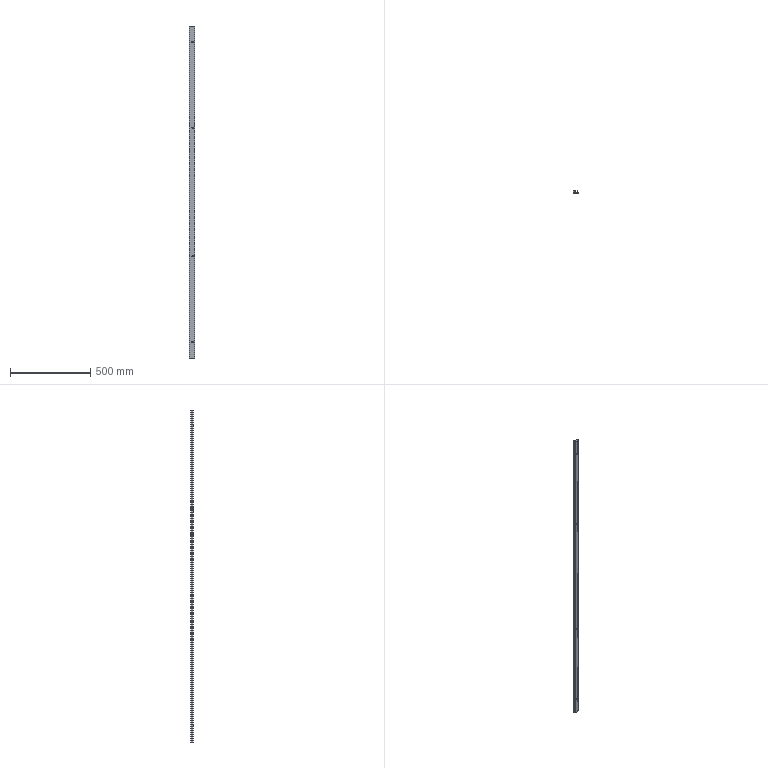Part | SolidWorks | features ICE 2, BaseBody 1, HoleWzd 1, MoveFace 1 | 1 solid | 35 faces | box 33.5 x 13.5 x 2066 mm | volume 386658 mm3 | plane 17 | cylinder 10 | cone 8 | commonest cylinder face diameters 13.44 x4 2 x3 4 x2 1.5 x1
STEP:
#1=CARTESIAN_POINT('',(20.,0.,1869.72));
#2=VERTEX_POINT('',#1);
#3=CARTESIAN_POINT('',(20.,0.,1862.28));
#4=VERTEX_POINT('',#3);
#5=CARTESIAN_POINT('',(20.,0.,1866.));
#6=DIRECTION('',(0.,-1.,0.));
#7=DIRECTION('',(0.,0.,-1.));
#8=AXIS2_PLACEMENT_3D('',#5,#6,#7);
#9=CIRCLE('',#8,3.72);
#10=EDGE_CURVE('',#2,#4,#9,.T.);
#11=ORIENTED_EDGE('',*,*,#10,.T.);
#12=CARTESIAN_POINT('',(20.,3.,1859.28));
#13=VERTEX_POINT('',#12);
#14=CARTESIAN_POINT('',(20.,3.,1859.28));
#15=DIRECTION('',(0.,0.7071,-0.7071));
#16=VECTOR('',#15,1000.);
#17=LINE('',#14,#16);
#18=EDGE_CURVE('',#4,#13,#17,.T.);
#19=ORIENTED_EDGE('',*,*,#18,.T.);
#20=CARTESIAN_POINT('',(20.,3.,1872.72));
#21=VERTEX_POINT('',#20);
#22=CARTESIAN_POINT('',(20.,3.,1866.));
#23=DIRECTION('',(0.,1.,0.));
#24=DIRECTION('',(0.,0.,1.));
#25=AXIS2_PLACEMENT_3D('',#22,#23,#24);
#26=CIRCLE('',#25,6.72);
#27=EDGE_CURVE('',#13,#21,#26,.T.);
#28=ORIENTED_EDGE('',*,*,#27,.T.);
#29=CARTESIAN_POINT('',(20.,3.,1872.72));
#30=DIRECTION('',(0.,0.7071,0.7071));
#31=VECTOR('',#30,1000.);
#32=LINE('',#29,#31);
#33=EDGE_CURVE('',#2,#21,#32,.T.);
#34=ORIENTED_EDGE('',*,*,#33,.F.);
#35=EDGE_LOOP('',(#11,#19,#28,#34));
#36=FACE_OUTER_BOUND('',#35,.T.);
#37=CARTESIAN_POINT('',(20.,3.,1866.));
#38=DIRECTION('',(0.,1.,0.));
#39=DIRECTION('',(0.,0.,1.));
#40=AXIS2_PLACEMENT_3D('',#37,#38,#39);
#41=CONICAL_SURFACE('',#40,6.72,0.7854);
#42=ADVANCED_FACE('',(#36),#41,.F.);
#43=CARTESIAN_POINT('',(20.,0.,3.72));
#44=VERTEX_POINT('',#43);
#45=CARTESIAN_POINT('',(20.,0.,-3.72));
#46=VERTEX_POINT('',#45);
#47=CARTESIAN_POINT('',(20.,0.,0.));
#48=DIRECTION('',(0.,-1.,0.));
#49=DIRECTION('',(0.,0.,-1.));
#50=AXIS2_PLACEMENT_3D('',#47,#48,#49);
#51=CIRCLE('',#50,3.72);
#52=EDGE_CURVE('',#44,#46,#51,.T.);
#53=ORIENTED_EDGE('',*,*,#52,.T.);
#54=CARTESIAN_POINT('',(20.,3.,-6.72));
#55=VERTEX_POINT('',#54);
#56=CARTESIAN_POINT('',(20.,3.,-6.72));
#57=DIRECTION('',(0.,0.7071,-0.7071));
#58=VECTOR('',#57,1000.);
#59=LINE('',#56,#58);
#60=EDGE_CURVE('',#46,#55,#59,.T.);
#61=ORIENTED_EDGE('',*,*,#60,.T.);
#62=CARTESIAN_POINT('',(20.,3.,6.72));
#63=VERTEX_POINT('',#62);
#64=CARTESIAN_POINT('',(20.,3.,0.));
#65=DIRECTION('',(0.,1.,0.));
#66=DIRECTION('',(0.,0.,1.));
#67=AXIS2_PLACEMENT_3D('',#64,#65,#66);
#68=CIRCLE('',#67,6.72);
#69=EDGE_CURVE('',#55,#63,#68,.T.);
#70=ORIENTED_EDGE('',*,*,#69,.T.);
#71=CARTESIAN_POINT('',(20.,3.,6.72));
#72=DIRECTION('',(0.,0.7071,0.7071));
#73=VECTOR('',#72,1000.);
#74=LINE('',#71,#73);
#75=EDGE_CURVE('',#44,#63,#74,.T.);
#76=ORIENTED_EDGE('',*,*,#75,.F.);
#77=EDGE_LOOP('',(#53,#61,#70,#76));
#78=FACE_OUTER_BOUND('',#77,.T.);
#79=CARTESIAN_POINT('',(20.,3.,0.));
#80=DIRECTION('',(0.,1.,0.));
#81=DIRECTION('',(0.,0.,1.));
#82=AXIS2_PLACEMENT_3D('',#79,#80,#81);
#83=CONICAL_SURFACE('',#82,6.72,0.7854);
#84=ADVANCED_FACE('',(#78),#83,.F.);
#85=CARTESIAN_POINT('',(20.,0.,536.72));
#86=VERTEX_POINT('',#85);
#87=CARTESIAN_POINT('',(20.,0.,529.28));
#88=VERTEX_POINT('',#87);
#89=CARTESIAN_POINT('',(20.,0.,533.));
#90=DIRECTION('',(0.,-1.,0.));
#91=DIRECTION('',(0.,0.,-1.));
#92=AXIS2_PLACEMENT_3D('',#89,#90,#91);
#93=CIRCLE('',#92,3.72);
#94=EDGE_CURVE('',#86,#88,#93,.T.);
#95=ORIENTED_EDGE('',*,*,#94,.T.);
#96=CARTESIAN_POINT('',(20.,3.,526.28));
#97=VERTEX_POINT('',#96);
#98=CARTESIAN_POINT('',(20.,3.,526.28));
#99=DIRECTION('',(0.,0.7071,-0.7071));
#100=VECTOR('',#99,1000.);
#101=LINE('',#98,#100);
#102=EDGE_CURVE('',#88,#97,#101,.T.);
#103=ORIENTED_EDGE('',*,*,#102,.T.);
#104=CARTESIAN_POINT('',(20.,3.,539.72));
#105=VERTEX_POINT('',#104);
#106=CARTESIAN_POINT('',(20.,3.,533.));
#107=DIRECTION('',(0.,1.,0.));
#108=DIRECTION('',(0.,0.,1.));
#109=AXIS2_PLACEMENT_3D('',#106,#107,#108);
#110=CIRCLE('',#109,6.72);
#111=EDGE_CURVE('',#97,#105,#110,.T.);
#112=ORIENTED_EDGE('',*,*,#111,.T.);
#113=CARTESIAN_POINT('',(20.,3.,539.72));
#114=DIRECTION('',(0.,0.7071,0.7071));
#115=VECTOR('',#114,1000.);
#116=LINE('',#113,#115);
#117=EDGE_CURVE('',#86,#105,#116,.T.);
#118=ORIENTED_EDGE('',*,*,#117,.F.);
#119=EDGE_LOOP('',(#95,#103,#112,#118));
#120=FACE_OUTER_BOUND('',#119,.T.);
#121=CARTESIAN_POINT('',(20.,3.,533.));
#122=DIRECTION('',(0.,1.,0.));
#123=DIRECTION('',(0.,0.,1.));
#124=AXIS2_PLACEMENT_3D('',#121,#122,#123);
#125=CONICAL_SURFACE('',#124,6.72,0.7854);
#126=ADVANCED_FACE('',(#120),#125,.F.);
#127=CARTESIAN_POINT('',(20.,0.,1336.72));
#128=VERTEX_POINT('',#127);
#129=CARTESIAN_POINT('',(20.,0.,1329.28));
#130=VERTEX_POINT('',#129);
#131=CARTESIAN_POINT('',(20.,0.,1333.));
#132=DIRECTION('',(0.,-1.,0.));
#133=DIRECTION('',(0.,0.,-1.));
#134=AXIS2_PLACEMENT_3D('',#131,#132,#133);
#135=CIRCLE('',#134,3.72);
#136=EDGE_CURVE('',#128,#130,#135,.T.);
#137=ORIENTED_EDGE('',*,*,#136,.T.);
#138=CARTESIAN_POINT('',(20.,3.,1326.28));
#139=VERTEX_POINT('',#138);
#140=CARTESIAN_POINT('',(20.,3.,1326.28));
#141=DIRECTION('',(0.,0.7071,-0.7071));
#142=VECTOR('',#141,1000.);
#143=LINE('',#140,#142);
#144=EDGE_CURVE('',#130,#139,#143,.T.);
#145=ORIENTED_EDGE('',*,*,#144,.T.);
#146=CARTESIAN_POINT('',(20.,3.,1339.72));
#147=VERTEX_POINT('',#146);
#148=CARTESIAN_POINT('',(20.,3.,1333.));
#149=DIRECTION('',(0.,1.,0.));
#150=DIRECTION('',(0.,0.,1.));
#151=AXIS2_PLACEMENT_3D('',#148,#149,#150);
#152=CIRCLE('',#151,6.72);
#153=EDGE_CURVE('',#139,#147,#152,.T.);
#154=ORIENTED_EDGE('',*,*,#153,.T.);
#155=CARTESIAN_POINT('',(20.,3.,1339.72));
#156=DIRECTION('',(0.,0.7071,0.7071));
#157=VECTOR('',#156,1000.);
#158=LINE('',#155,#157);
#159=EDGE_CURVE('',#128,#147,#158,.T.);
#160=ORIENTED_EDGE('',*,*,#159,.F.);
#161=EDGE_LOOP('',(#137,#145,#154,#160));
#162=FACE_OUTER_BOUND('',#161,.T.);
#163=CARTESIAN_POINT('',(20.,3.,1333.));
#164=DIRECTION('',(0.,1.,0.));
#165=DIRECTION('',(0.,0.,1.));
#166=AXIS2_PLACEMENT_3D('',#163,#164,#165);
#167=CONICAL_SURFACE('',#166,6.72,0.7854);
#168=ADVANCED_FACE('',(#162),#167,.F.);
#169=CARTESIAN_POINT('',(24.5,10.5,1328.009));
#170=VERTEX_POINT('',#169);
#171=CARTESIAN_POINT('',(24.5,3.,1328.009));
#172=VERTEX_POINT('',#171);
#173=CARTESIAN_POINT('',(24.5,64.,1328.009));
#174=DIRECTION('',(0.,-1.,0.));
#175=VECTOR('',#174,1000.);
#176=LINE('',#173,#175);
#177=EDGE_CURVE('',#170,#172,#176,.T.);
#178=ORIENTED_EDGE('',*,*,#177,.F.);
#179=CARTESIAN_POINT('',(24.5,10.5,537.991));
#180=VERTEX_POINT('',#179);
#181=CARTESIAN_POINT('',(24.5,10.5,-100.));
#182=DIRECTION('',(0.,0.,-1.));
#183=VECTOR('',#182,1000.);
#184=LINE('',#181,#183);
#185=EDGE_CURVE('',#170,#180,#184,.T.);
#186=ORIENTED_EDGE('',*,*,#185,.T.);
#187=CARTESIAN_POINT('',(24.5,3.,537.991));
#188=VERTEX_POINT('',#187);
#189=CARTESIAN_POINT('',(24.5,13.5,537.991));
#190=DIRECTION('',(0.,-1.,0.));
#191=VECTOR('',#190,1000.);
#192=LINE('',#189,#191);
#193=EDGE_CURVE('',#180,#188,#192,.T.);
#194=ORIENTED_EDGE('',*,*,#193,.T.);
#195=CARTESIAN_POINT('',(24.5,3.,-100.));
#196=DIRECTION('',(0.,0.,-1.));
#197=VECTOR('',#196,1000.);
#198=LINE('',#195,#197);
#199=EDGE_CURVE('',#172,#188,#198,.T.);
#200=ORIENTED_EDGE('',*,*,#199,.F.);
#201=EDGE_LOOP('',(#178,#186,#194,#200));
#202=FACE_OUTER_BOUND('',#201,.T.);
#203=CARTESIAN_POINT('',(24.5,10.5,-100.));
#204=DIRECTION('',(-1.,0.,0.));
#205=DIRECTION('',(0.,0.,1.));
#206=AXIS2_PLACEMENT_3D('',#203,#204,#205);
#207=PLANE('',#206);
#208=ADVANCED_FACE('',(#202),#207,.T.);
#209=CARTESIAN_POINT('',(24.5,10.5,1337.991));
#210=VERTEX_POINT('',#209);
#211=CARTESIAN_POINT('',(24.5,10.5,1337.991));
#212=CARTESIAN_POINT('',(24.5,10.64,1337.991));
#213=CARTESIAN_POINT('',(24.514,10.776,1337.978));
#214=CARTESIAN_POINT('',(24.57,11.042,1337.927));
#215=CARTESIAN_POINT('',(24.611,11.171,1337.889));
#216=CARTESIAN_POINT('',(24.713,11.408,1337.791));
#217=CARTESIAN_POINT('',(24.775,11.519,1337.73));
#218=CARTESIAN_POINT('',(24.908,11.717,1337.591));
#219=CARTESIAN_POINT('',(24.981,11.806,1337.512));
#220=CARTESIAN_POINT('',(25.207,12.042,1337.254));
#221=CARTESIAN_POINT('',(25.363,12.155,1337.058));
#222=CARTESIAN_POINT('',(25.665,12.326,1336.624));
#223=CARTESIAN_POINT('',(25.806,12.38,1336.395));
#224=CARTESIAN_POINT('',(26.061,12.456,1335.916));
#225=CARTESIAN_POINT('',(26.176,12.476,1335.663));
#226=CARTESIAN_POINT('',(26.372,12.498,1335.151));
#227=CARTESIAN_POINT('',(26.454,12.501,1334.891));
#228=CARTESIAN_POINT('',(26.586,12.499,1334.362));
#229=CARTESIAN_POINT('',(26.636,12.496,1334.093));
#230=CARTESIAN_POINT('',(26.703,12.49,1333.547));
#231=CARTESIAN_POINT('',(26.72,12.488,1333.271));
#232=CARTESIAN_POINT('',(26.72,12.488,1332.725));
#233=CARTESIAN_POINT('',(26.703,12.49,1332.453));
#234=CARTESIAN_POINT('',(26.637,12.496,1331.911));
#235=CARTESIAN_POINT('',(26.587,12.499,1331.64));
#236=CARTESIAN_POINT('',(26.387,12.501,1330.839));
#237=CARTESIAN_POINT('',(26.191,12.494,1330.329));
#238=CARTESIAN_POINT('',(25.805,12.38,1329.604));
#239=CARTESIAN_POINT('',(25.663,12.325,1329.373));
#240=CARTESIAN_POINT('',(25.364,12.155,1328.943));
#241=CARTESIAN_POINT('',(25.205,12.039,1328.744));
#242=CARTESIAN_POINT('',(24.981,11.805,1328.488));
#243=CARTESIAN_POINT('',(24.907,11.716,1328.408));
#244=CARTESIAN_POINT('',(24.774,11.518,1328.27));
#245=CARTESIAN_POINT('',(24.714,11.409,1328.21));
#246=CARTESIAN_POINT('',(24.611,11.17,1328.111));
#247=CARTESIAN_POINT('',(24.571,11.044,1328.074));
#248=CARTESIAN_POINT('',(24.515,10.78,1328.023));
#249=CARTESIAN_POINT('',(24.5,10.64,1328.009));
#250=CARTESIAN_POINT('',(24.5,10.5,1328.009));
#251=B_SPLINE_CURVE_WITH_KNOTS('',3,(#211,#212,#213,#214,#215,#216,#217,#218,#219,#220,#221,#222,#223,#224,#225,#226,#227,#228,#229,#230,#231,#232,#233,#234,#235,#236,#237,#238,#239,#240,#241,#242,#243,#244,#245,#246,#247,#248,#249,#250),.UNSPECIFIED.,.F.,.F.,(4,2,2,2,2,2,2,2,2,2,2,2,2,2,2,2,2,2,2,4),(0.,0.0004127,0.0008255,0.001238,0.001651,0.002476,0.003302,0.004127,0.004953,0.005778,0.006604,0.007429,0.008255,0.009906,0.01073,0.01156,0.01197,0.01238,0.01279,0.01321),.UNSPECIFIED.);
#252=EDGE_CURVE('',#210,#170,#251,.T.);
#253=ORIENTED_EDGE('',*,*,#252,.F.);
#254=CARTESIAN_POINT('',(24.5,10.5,1861.009));
#255=VERTEX_POINT('',#254);
#256=CARTESIAN_POINT('',(24.5,10.5,-100.));
#257=DIRECTION('',(0.,0.,-1.));
#258=VECTOR('',#257,1000.);
#259=LINE('',#256,#258);
#260=EDGE_CURVE('',#255,#210,#259,.T.);
#261=ORIENTED_EDGE('',*,*,#260,.F.);
#262=CARTESIAN_POINT('',(24.5,10.5,1870.991));
#263=VERTEX_POINT('',#262);
#264=CARTESIAN_POINT('',(24.5,10.5,1861.009));
#265=CARTESIAN_POINT('',(24.5,10.64,1861.009));
#266=CARTESIAN_POINT('',(24.514,10.776,1861.022));
#267=CARTESIAN_POINT('',(24.57,11.042,1861.073));
#268=CARTESIAN_POINT('',(24.611,11.171,1861.111));
#269=CARTESIAN_POINT('',(24.713,11.408,1861.209));
#270=CARTESIAN_POINT('',(24.775,11.519,1861.27));
#271=CARTESIAN_POINT('',(24.908,11.717,1861.409));
#272=CARTESIAN_POINT('',(24.981,11.806,1861.488));
#273=CARTESIAN_POINT('',(25.207,12.042,1861.746));
#274=CARTESIAN_POINT('',(25.363,12.155,1861.942));
#275=CARTESIAN_POINT('',(25.665,12.326,1862.376));
#276=CARTESIAN_POINT('',(25.806,12.38,1862.605));
#277=CARTESIAN_POINT('',(26.061,12.456,1863.084));
#278=CARTESIAN_POINT('',(26.176,12.476,1863.337));
#279=CARTESIAN_POINT('',(26.372,12.498,1863.849));
#280=CARTESIAN_POINT('',(26.454,12.501,1864.109));
#281=CARTESIAN_POINT('',(26.586,12.499,1864.638));
#282=CARTESIAN_POINT('',(26.636,12.496,1864.907));
#283=CARTESIAN_POINT('',(26.703,12.49,1865.453));
#284=CARTESIAN_POINT('',(26.72,12.488,1865.729));
#285=CARTESIAN_POINT('',(26.72,12.488,1866.275));
#286=CARTESIAN_POINT('',(26.703,12.49,1866.547));
#287=CARTESIAN_POINT('',(26.637,12.496,1867.089));
#288=CARTESIAN_POINT('',(26.587,12.499,1867.36));
#289=CARTESIAN_POINT('',(26.387,12.501,1868.161));
#290=CARTESIAN_POINT('',(26.191,12.494,1868.671));
#291=CARTESIAN_POINT('',(25.805,12.38,1869.396));
#292=CARTESIAN_POINT('',(25.663,12.325,1869.627));
#293=CARTESIAN_POINT('',(25.364,12.155,1870.057));
#294=CARTESIAN_POINT('',(25.205,12.039,1870.256));
#295=CARTESIAN_POINT('',(24.981,11.805,1870.512));
#296=CARTESIAN_POINT('',(24.907,11.716,1870.592));
#297=CARTESIAN_POINT('',(24.774,11.518,1870.73));
#298=CARTESIAN_POINT('',(24.714,11.409,1870.79));
#299=CARTESIAN_POINT('',(24.611,11.17,1870.889));
#300=CARTESIAN_POINT('',(24.571,11.044,1870.926));
#301=CARTESIAN_POINT('',(24.515,10.78,1870.977));
#302=CARTESIAN_POINT('',(24.5,10.64,1870.991));
#303=CARTESIAN_POINT('',(24.5,10.5,1870.991));
#304=B_SPLINE_CURVE_WITH_KNOTS('',3,(#264,#265,#266,#267,#268,#269,#270,#271,#272,#273,#274,#275,#276,#277,#278,#279,#280,#281,#282,#283,#284,#285,#286,#287,#288,#289,#290,#291,#292,#293,#294,#295,#296,#297,#298,#299,#300,#301,#302,#303),.UNSPECIFIED.,.F.,.F.,(4,2,2,2,2,2,2,2,2,2,2,2,2,2,2,2,2,2,2,4),(0.,0.0004127,0.0008255,0.001238,0.001651,0.002476,0.003302,0.004127,0.004953,0.005778,0.006604,0.007429,0.008255,0.009906,0.01073,0.01156,0.01197,0.01238,0.01279,0.01321),.UNSPECIFIED.);
#305=EDGE_CURVE('',#255,#263,#304,.T.);
#306=ORIENTED_EDGE('',*,*,#305,.T.);
#307=CARTESIAN_POINT('',(24.5,10.5,1966.));
#308=VERTEX_POINT('',#307);
#309=CARTESIAN_POINT('',(24.5,10.5,-100.));
#310=DIRECTION('',(0.,0.,-1.));
#311=VECTOR('',#310,1000.);
#312=LINE('',#309,#311);
#313=EDGE_CURVE('',#308,#263,#312,.T.);
#314=ORIENTED_EDGE('',*,*,#313,.F.);
#315=CARTESIAN_POINT('',(28.5,10.5,1966.));
#316=VERTEX_POINT('',#315);
#317=CARTESIAN_POINT('',(26.5,10.5,1966.));
#318=DIRECTION('',(0.,0.,1.));
#319=DIRECTION('',(1.,0.,0.));
#320=AXIS2_PLACEMENT_3D('',#317,#318,#319);
#321=CIRCLE('',#320,2.);
#322=EDGE_CURVE('',#316,#308,#321,.T.);
#323=ORIENTED_EDGE('',*,*,#322,.F.);
#324=CARTESIAN_POINT('',(28.5,10.5,-100.));
#325=VERTEX_POINT('',#324);
#326=CARTESIAN_POINT('',(28.5,10.5,-100.));
#327=DIRECTION('',(0.,0.,-1.));
#328=VECTOR('',#327,1000.);
#329=LINE('',#326,#328);
#330=EDGE_CURVE('',#316,#325,#329,.T.);
#331=ORIENTED_EDGE('',*,*,#330,.T.);
#332=CARTESIAN_POINT('',(24.5,10.5,-100.));
#333=VERTEX_POINT('',#332);
#334=CARTESIAN_POINT('',(26.5,10.5,-100.));
#335=DIRECTION('',(0.,0.,1.));
#336=DIRECTION('',(-1.,0.,0.));
#337=AXIS2_PLACEMENT_3D('',#334,#335,#336);
#338=CIRCLE('',#337,2.);
#339=EDGE_CURVE('',#325,#333,#338,.T.);
#340=ORIENTED_EDGE('',*,*,#339,.T.);
#341=CARTESIAN_POINT('',(24.5,10.5,-4.991));
#342=VERTEX_POINT('',#341);
#343=CARTESIAN_POINT('',(24.5,10.5,-100.));
#344=DIRECTION('',(0.,0.,-1.));
#345=VECTOR('',#344,1000.);
#346=LINE('',#343,#345);
#347=EDGE_CURVE('',#342,#333,#346,.T.);
#348=ORIENTED_EDGE('',*,*,#347,.F.);
#349=CARTESIAN_POINT('',(24.5,10.5,4.991));
#350=VERTEX_POINT('',#349);
#351=CARTESIAN_POINT('',(24.5,10.5,-4.991));
#352=CARTESIAN_POINT('',(24.5,10.638,-4.991));
#353=CARTESIAN_POINT('',(24.515,10.777,-4.978));
#354=CARTESIAN_POINT('',(24.57,11.043,-4.927));
#355=CARTESIAN_POINT('',(24.611,11.171,-4.889));
#356=CARTESIAN_POINT('',(24.765,11.529,-4.74));
#357=CARTESIAN_POINT('',(24.907,11.728,-4.597));
#358=CARTESIAN_POINT('',(25.205,12.04,-4.256));
#359=CARTESIAN_POINT('',(25.365,12.156,-4.055));
#360=CARTESIAN_POINT('',(25.663,12.325,-3.627));
#361=CARTESIAN_POINT('',(25.806,12.38,-3.395));
#362=CARTESIAN_POINT('',(26.19,12.494,-2.672));
#363=CARTESIAN_POINT('',(26.387,12.501,-2.161));
#364=CARTESIAN_POINT('',(26.654,12.499,-1.091));
#365=CARTESIAN_POINT('',(26.72,12.488,-0.5481));
#366=CARTESIAN_POINT('',(26.72,12.488,0.2773));
#367=CARTESIAN_POINT('',(26.703,12.49,0.5529));
#368=CARTESIAN_POINT('',(26.636,12.496,1.095));
#369=CARTESIAN_POINT('',(26.586,12.499,1.362));
#370=CARTESIAN_POINT('',(26.388,12.501,2.155));
#371=CARTESIAN_POINT('',(26.188,12.493,2.677));
#372=CARTESIAN_POINT('',(25.805,12.38,3.396));
#373=CARTESIAN_POINT('',(25.662,12.324,3.629));
#374=CARTESIAN_POINT('',(25.438,12.197,3.95));
#375=CARTESIAN_POINT('',(25.362,12.147,4.053));
#376=CARTESIAN_POINT('',(25.208,12.03,4.249));
#377=CARTESIAN_POINT('',(25.13,11.961,4.342));
#378=CARTESIAN_POINT('',(24.98,11.805,4.513));
#379=CARTESIAN_POINT('',(24.908,11.717,4.591));
#380=CARTESIAN_POINT('',(24.774,11.518,4.73));
#381=CARTESIAN_POINT('',(24.714,11.408,4.79));
#382=CARTESIAN_POINT('',(24.612,11.172,4.888));
#383=CARTESIAN_POINT('',(24.57,11.043,4.927));
#384=CARTESIAN_POINT('',(24.515,10.778,4.978));
#385=CARTESIAN_POINT('',(24.5,10.64,4.991));
#386=CARTESIAN_POINT('',(24.5,10.5,4.991));
#387=B_SPLINE_CURVE_WITH_KNOTS('',3,(#351,#352,#353,#354,#355,#356,#357,#358,#359,#360,#361,#362,#363,#364,#365,#366,#367,#368,#369,#370,#371,#372,#373,#374,#375,#376,#377,#378,#379,#380,#381,#382,#383,#384,#385,#386),.UNSPECIFIED.,.F.,.F.,(4,2,2,2,2,2,2,2,2,2,2,2,2,2,2,2,2,4),(0.01321,0.01362,0.01403,0.01486,0.01569,0.01651,0.01816,0.01981,0.02064,0.02146,0.02311,0.02394,0.02435,0.02477,0.02518,0.02559,0.026,0.02642),.UNSPECIFIED.);
#388=EDGE_CURVE('',#342,#350,#387,.T.);
#389=ORIENTED_EDGE('',*,*,#388,.T.);
#390=CARTESIAN_POINT('',(24.5,10.5,528.009));
#391=VERTEX_POINT('',#390);
#392=CARTESIAN_POINT('',(24.5,10.5,-100.));
#393=DIRECTION('',(0.,0.,-1.));
#394=VECTOR('',#393,1000.);
#395=LINE('',#392,#394);
#396=EDGE_CURVE('',#391,#350,#395,.T.);
#397=ORIENTED_EDGE('',*,*,#396,.F.);
#398=CARTESIAN_POINT('',(24.5,10.5,528.009));
#399=CARTESIAN_POINT('',(24.5,10.638,528.009));
#400=CARTESIAN_POINT('',(24.515,10.777,528.022));
#401=CARTESIAN_POINT('',(24.57,11.043,528.073));
#402=CARTESIAN_POINT('',(24.611,11.171,528.111));
#403=CARTESIAN_POINT('',(24.765,11.529,528.26));
#404=CARTESIAN_POINT('',(24.907,11.728,528.403));
#405=CARTESIAN_POINT('',(25.205,12.04,528.744));
#406=CARTESIAN_POINT('',(25.365,12.156,528.945));
#407=CARTESIAN_POINT('',(25.663,12.325,529.373));
#408=CARTESIAN_POINT('',(25.806,12.38,529.605));
#409=CARTESIAN_POINT('',(26.19,12.494,530.328));
#410=CARTESIAN_POINT('',(26.387,12.501,530.839));
#411=CARTESIAN_POINT('',(26.654,12.499,531.909));
#412=CARTESIAN_POINT('',(26.72,12.488,532.452));
#413=CARTESIAN_POINT('',(26.72,12.488,533.277));
#414=CARTESIAN_POINT('',(26.703,12.49,533.553));
#415=CARTESIAN_POINT('',(26.636,12.496,534.095));
#416=CARTESIAN_POINT('',(26.586,12.499,534.362));
#417=CARTESIAN_POINT('',(26.388,12.501,535.155));
#418=CARTESIAN_POINT('',(26.188,12.493,535.677));
#419=CARTESIAN_POINT('',(25.805,12.38,536.396));
#420=CARTESIAN_POINT('',(25.662,12.324,536.629));
#421=CARTESIAN_POINT('',(25.438,12.197,536.95));
#422=CARTESIAN_POINT('',(25.362,12.147,537.053));
#423=CARTESIAN_POINT('',(25.208,12.03,537.249));
#424=CARTESIAN_POINT('',(25.13,11.961,537.342));
#425=CARTESIAN_POINT('',(24.98,11.805,537.513));
#426=CARTESIAN_POINT('',(24.908,11.717,537.591));
#427=CARTESIAN_POINT('',(24.774,11.518,537.73));
#428=CARTESIAN_POINT('',(24.714,11.408,537.79));
#429=CARTESIAN_POINT('',(24.612,11.172,537.888));
#430=CARTESIAN_POINT('',(24.57,11.043,537.927));
#431=CARTESIAN_POINT('',(24.515,10.778,537.978));
#432=CARTESIAN_POINT('',(24.5,10.64,537.991));
#433=CARTESIAN_POINT('',(24.5,10.5,537.991));
#434=B_SPLINE_CURVE_WITH_KNOTS('',3,(#398,#399,#400,#401,#402,#403,#404,#405,#406,#407,#408,#409,#410,#411,#412,#413,#414,#415,#416,#417,#418,#419,#420,#421,#422,#423,#424,#425,#426,#427,#428,#429,#430,#431,#432,#433),.UNSPECIFIED.,.F.,.F.,(4,2,2,2,2,2,2,2,2,2,2,2,2,2,2,2,2,4),(0.01321,0.01362,0.01403,0.01486,0.01569,0.01651,0.01816,0.01981,0.02064,0.02146,0.02311,0.02394,0.02435,0.02477,0.02518,0.02559,0.026,0.02642),.UNSPECIFIED.);
#435=EDGE_CURVE('',#391,#180,#434,.T.);
#436=ORIENTED_EDGE('',*,*,#435,.T.);
#437=ORIENTED_EDGE('',*,*,#185,.F.);
#438=EDGE_LOOP('',(#253,#261,#306,#314,#323,#331,#340,#348,#389,#397,#436,#437));
#439=FACE_OUTER_BOUND('',#438,.T.);
#440=CARTESIAN_POINT('',(26.5,10.5,-100.));
#441=DIRECTION('',(0.,0.,-1.));
#442=DIRECTION('',(-1.,0.,0.));
#443=AXIS2_PLACEMENT_3D('',#440,#441,#442);
#444=CYLINDRICAL_SURFACE('',#443,2.);
#445=ADVANCED_FACE('',(#439),#444,.T.);
#446=CARTESIAN_POINT('',(24.5,3.,-4.991));
#447=VERTEX_POINT('',#446);
#448=CARTESIAN_POINT('',(24.5,3.,-100.));
#449=VERTEX_POINT('',#448);
#450=CARTESIAN_POINT('',(24.5,3.,-100.));
#451=DIRECTION('',(0.,0.,-1.));
#452=VECTOR('',#451,1000.);
#453=LINE('',#450,#452);
#454=EDGE_CURVE('',#447,#449,#453,.T.);
#455=ORIENTED_EDGE('',*,*,#454,.F.);
#456=CARTESIAN_POINT('',(24.5,13.5,-4.991));
#457=DIRECTION('',(0.,1.,0.));
#458=VECTOR('',#457,1000.);
#459=LINE('',#456,#458);
#460=EDGE_CURVE('',#447,#342,#459,.T.);
#461=ORIENTED_EDGE('',*,*,#460,.T.);
#462=ORIENTED_EDGE('',*,*,#347,.T.);
#463=CARTESIAN_POINT('',(24.5,1.,-100.));
#464=DIRECTION('',(0.,-1.,0.));
#465=VECTOR('',#464,1000.);
#466=LINE('',#463,#465);
#467=EDGE_CURVE('',#333,#449,#466,.T.);
#468=ORIENTED_EDGE('',*,*,#467,.T.);
#469=EDGE_LOOP('',(#455,#461,#462,#468));
#470=FACE_OUTER_BOUND('',#469,.T.);
#471=CARTESIAN_POINT('',(24.5,10.5,-100.));
#472=DIRECTION('',(-1.,0.,0.));
#473=DIRECTION('',(0.,0.,1.));
#474=AXIS2_PLACEMENT_3D('',#471,#472,#473);
#475=PLANE('',#474);
#476=ADVANCED_FACE('',(#470),#475,.T.);
#477=ORIENTED_EDGE('',*,*,#396,.T.);
#478=CARTESIAN_POINT('',(24.5,3.,4.991));
#479=VERTEX_POINT('',#478);
#480=CARTESIAN_POINT('',(24.5,13.5,4.991));
#481=DIRECTION('',(0.,-1.,0.));
#482=VECTOR('',#481,1000.);
#483=LINE('',#480,#482);
#484=EDGE_CURVE('',#350,#479,#483,.T.);
#485=ORIENTED_EDGE('',*,*,#484,.T.);
#486=CARTESIAN_POINT('',(24.5,3.,528.009));
#487=VERTEX_POINT('',#486);
#488=CARTESIAN_POINT('',(24.5,3.,-100.));
#489=DIRECTION('',(0.,0.,-1.));
#490=VECTOR('',#489,1000.);
#491=LINE('',#488,#490);
#492=EDGE_CURVE('',#487,#479,#491,.T.);
#493=ORIENTED_EDGE('',*,*,#492,.F.);
#494=CARTESIAN_POINT('',(24.5,13.5,528.009));
#495=DIRECTION('',(0.,1.,0.));
#496=VECTOR('',#495,1000.);
#497=LINE('',#494,#496);
#498=EDGE_CURVE('',#487,#391,#497,.T.);
#499=ORIENTED_EDGE('',*,*,#498,.T.);
#500=EDGE_LOOP('',(#477,#485,#493,#499));
#501=FACE_OUTER_BOUND('',#500,.T.);
#502=CARTESIAN_POINT('',(24.5,10.5,-100.));
#503=DIRECTION('',(-1.,0.,0.));
#504=DIRECTION('',(0.,0.,1.));
#505=AXIS2_PLACEMENT_3D('',#502,#503,#504);
#506=PLANE('',#505);
#507=ADVANCED_FACE('',(#501),#506,.T.);
#508=CARTESIAN_POINT('',(24.5,3.,1337.991));
#509=VERTEX_POINT('',#508);
#510=CARTESIAN_POINT('',(24.5,64.,1337.991));
#511=DIRECTION('',(0.,1.,0.));
#512=VECTOR('',#511,1000.);
#513=LINE('',#510,#512);
#514=EDGE_CURVE('',#509,#210,#513,.T.);
#515=ORIENTED_EDGE('',*,*,#514,.F.);
#516=CARTESIAN_POINT('',(24.5,3.,1861.009));
#517=VERTEX_POINT('',#516);
#518=CARTESIAN_POINT('',(24.5,3.,-100.));
#519=DIRECTION('',(0.,0.,-1.));
#520=VECTOR('',#519,1000.);
#521=LINE('',#518,#520);
#522=EDGE_CURVE('',#517,#509,#521,.T.);
#523=ORIENTED_EDGE('',*,*,#522,.F.);
#524=CARTESIAN_POINT('',(24.5,13.5,1861.009));
#525=DIRECTION('',(0.,1.,0.));
#526=VECTOR('',#525,1000.);
#527=LINE('',#524,#526);
#528=EDGE_CURVE('',#517,#255,#527,.T.);
#529=ORIENTED_EDGE('',*,*,#528,.T.);
#530=ORIENTED_EDGE('',*,*,#260,.T.);
#531=EDGE_LOOP('',(#515,#523,#529,#530));
#532=FACE_OUTER_BOUND('',#531,.T.);
#533=CARTESIAN_POINT('',(24.5,10.5,-100.));
#534=DIRECTION('',(-1.,0.,0.));
#535=DIRECTION('',(0.,0.,1.));
#536=AXIS2_PLACEMENT_3D('',#533,#534,#535);
#537=PLANE('',#536);
#538=ADVANCED_FACE('',(#532),#537,.T.);
#539=ORIENTED_EDGE('',*,*,#313,.T.);
#540=CARTESIAN_POINT('',(24.5,3.,1870.991));
#541=VERTEX_POINT('',#540);
#542=CARTESIAN_POINT('',(24.5,13.5,1870.991));
#543=DIRECTION('',(0.,-1.,0.));
#544=VECTOR('',#543,1000.);
#545=LINE('',#542,#544);
#546=EDGE_CURVE('',#263,#541,#545,.T.);
#547=ORIENTED_EDGE('',*,*,#546,.T.);
#548=CARTESIAN_POINT('',(24.5,3.,1966.));
#549=VERTEX_POINT('',#548);
#550=CARTESIAN_POINT('',(24.5,3.,-100.));
#551=DIRECTION('',(0.,0.,-1.));
#552=VECTOR('',#551,1000.);
#553=LINE('',#550,#552);
#554=EDGE_CURVE('',#549,#541,#553,.T.);
#555=ORIENTED_EDGE('',*,*,#554,.F.);
#556=CARTESIAN_POINT('',(24.5,1.,1966.));
#557=DIRECTION('',(0.,-1.,0.));
#558=VECTOR('',#557,1000.);
#559=LINE('',#556,#558);
#560=EDGE_CURVE('',#308,#549,#559,.T.);
#561=ORIENTED_EDGE('',*,*,#560,.F.);
#562=EDGE_LOOP('',(#539,#547,#555,#561));
#563=FACE_OUTER_BOUND('',#562,.T.);
#564=CARTESIAN_POINT('',(24.5,10.5,-100.));
#565=DIRECTION('',(-1.,0.,0.));
#566=DIRECTION('',(0.,0.,1.));
#567=AXIS2_PLACEMENT_3D('',#564,#565,#566);
#568=PLANE('',#567);
#569=ADVANCED_FACE('',(#563),#568,.T.);
#570=ORIENTED_EDGE('',*,*,#10,.F.);
#571=CARTESIAN_POINT('',(20.,0.,1866.));
#572=DIRECTION('',(0.,-1.,0.));
#573=DIRECTION('',(0.,0.,-1.));
#574=AXIS2_PLACEMENT_3D('',#571,#572,#573);
#575=CIRCLE('',#574,3.72);
#576=EDGE_CURVE('',#4,#2,#575,.T.);
#577=ORIENTED_EDGE('',*,*,#576,.F.);
#578=EDGE_LOOP('',(#570,#577));
#579=FACE_BOUND('',#578,.T.);
#580=ORIENTED_EDGE('',*,*,#94,.F.);
#581=CARTESIAN_POINT('',(20.,0.,533.));
#582=DIRECTION('',(0.,-1.,0.));
#583=DIRECTION('',(0.,0.,-1.));
#584=AXIS2_PLACEMENT_3D('',#581,#582,#583);
#585=CIRCLE('',#584,3.72);
#586=EDGE_CURVE('',#88,#86,#585,.T.);
#587=ORIENTED_EDGE('',*,*,#586,.F.);
#588=EDGE_LOOP('',(#580,#587));
#589=FACE_BOUND('',#588,.T.);
#590=ORIENTED_EDGE('',*,*,#136,.F.);
#591=CARTESIAN_POINT('',(20.,0.,1333.));
#592=DIRECTION('',(0.,-1.,0.));
#593=DIRECTION('',(0.,0.,-1.));
#594=AXIS2_PLACEMENT_3D('',#591,#592,#593);
#595=CIRCLE('',#594,3.72);
#596=EDGE_CURVE('',#130,#128,#595,.T.);
#597=ORIENTED_EDGE('',*,*,#596,.F.);
#598=EDGE_LOOP('',(#590,#597));
#599=FACE_BOUND('',#598,.T.);
#600=CARTESIAN_POINT('',(1.,0.,-100.));
#601=VERTEX_POINT('',#600);
#602=CARTESIAN_POINT('',(32.5,0.,-100.));
#603=VERTEX_POINT('',#602);
#604=CARTESIAN_POINT('',(1.,0.,-100.));
#605=DIRECTION('',(1.,0.,0.));
#606=VECTOR('',#605,1000.);
#607=LINE('',#604,#606);
#608=EDGE_CURVE('',#601,#603,#607,.T.);
#609=ORIENTED_EDGE('',*,*,#608,.T.);
#610=CARTESIAN_POINT('',(32.5,0.,1966.));
#611=VERTEX_POINT('',#610);
#612=CARTESIAN_POINT('',(32.5,0.,-100.));
#613=DIRECTION('',(0.,0.,1.));
#614=VECTOR('',#613,1000.);
#615=LINE('',#612,#614);
#616=EDGE_CURVE('',#603,#611,#615,.T.);
#617=ORIENTED_EDGE('',*,*,#616,.T.);
#618=CARTESIAN_POINT('',(1.,0.,1966.));
#619=VERTEX_POINT('',#618);
#620=CARTESIAN_POINT('',(1.,0.,1966.));
#621=DIRECTION('',(-1.,0.,0.));
#622=VECTOR('',#621,1000.);
#623=LINE('',#620,#622);
#624=EDGE_CURVE('',#611,#619,#623,.T.);
#625=ORIENTED_EDGE('',*,*,#624,.T.);
#626=CARTESIAN_POINT('',(1.,0.,-100.));
#627=DIRECTION('',(0.,0.,-1.));
#628=VECTOR('',#627,1000.);
#629=LINE('',#626,#628);
#630=EDGE_CURVE('',#619,#601,#629,.T.);
#631=ORIENTED_EDGE('',*,*,#630,.T.);
#632=EDGE_LOOP('',(#609,#617,#625,#631));
#633=FACE_OUTER_BOUND('',#632,.T.);
#634=ORIENTED_EDGE('',*,*,#52,.F.);
#635=CARTESIAN_POINT('',(20.,0.,0.));
#636=DIRECTION('',(0.,-1.,0.));
#637=DIRECTION('',(0.,0.,-1.));
#638=AXIS2_PLACEMENT_3D('',#635,#636,#637);
#639=CIRCLE('',#638,3.72);
#640=EDGE_CURVE('',#46,#44,#639,.T.);
#641=ORIENTED_EDGE('',*,*,#640,.F.);
#642=EDGE_LOOP('',(#634,#641));
#643=FACE_BOUND('',#642,.T.);
#644=CARTESIAN_POINT('',(1.,0.,-100.));
#645=DIRECTION('',(0.,-1.,0.));
#646=DIRECTION('',(0.,0.,-1.));
#647=AXIS2_PLACEMENT_3D('',#644,#645,#646);
#648=PLANE('',#647);
#649=ADVANCED_FACE('',(#579,#589,#599,#633,#643),#648,.T.);
#650=CARTESIAN_POINT('',(33.5,1.,-100.));
#651=VERTEX_POINT('',#650);
#652=CARTESIAN_POINT('',(32.5,1.,-100.));
#653=DIRECTION('',(0.,0.,1.));
#654=DIRECTION('',(-1.,0.,0.));
#655=AXIS2_PLACEMENT_3D('',#652,#653,#654);
#656=CIRCLE('',#655,1.);
#657=EDGE_CURVE('',#603,#651,#656,.T.);
#658=ORIENTED_EDGE('',*,*,#657,.T.);
#659=CARTESIAN_POINT('',(33.5,1.,1966.));
#660=VERTEX_POINT('',#659);
#661=CARTESIAN_POINT('',(33.5,1.,-100.));
#662=DIRECTION('',(0.,0.,1.));
#663=VECTOR('',#662,1000.);
#664=LINE('',#661,#663);
#665=EDGE_CURVE('',#651,#660,#664,.T.);
#666=ORIENTED_EDGE('',*,*,#665,.T.);
#667=CARTESIAN_POINT('',(32.5,1.,1966.));
#668=DIRECTION('',(0.,0.,-1.));
#669=DIRECTION('',(1.,0.,0.));
#670=AXIS2_PLACEMENT_3D('',#667,#668,#669);
#671=CIRCLE('',#670,1.);
#672=EDGE_CURVE('',#660,#611,#671,.T.);
#673=ORIENTED_EDGE('',*,*,#672,.T.);
#674=ORIENTED_EDGE('',*,*,#616,.F.);
#675=EDGE_LOOP('',(#658,#666,#673,#674));
#676=FACE_OUTER_BOUND('',#675,.T.);
#677=CARTESIAN_POINT('',(32.5,1.,-100.));
#678=DIRECTION('',(0.,0.,-1.));
#679=DIRECTION('',(-1.,0.,0.));
#680=AXIS2_PLACEMENT_3D('',#677,#678,#679);
#681=CYLINDRICAL_SURFACE('',#680,1.);
#682=ADVANCED_FACE('',(#676),#681,.T.);
#683=CARTESIAN_POINT('',(1.5,12.75,-100.));
#684=VERTEX_POINT('',#683);
#685=CARTESIAN_POINT('',(0.,12.75,-100.));
#686=VERTEX_POINT('',#685);
#687=CARTESIAN_POINT('',(0.75,12.75,-100.));
#688=DIRECTION('',(0.,0.,1.));
#689=DIRECTION('',(-1.,0.,0.));
#690=AXIS2_PLACEMENT_3D('',#687,#688,#689);
#691=CIRCLE('',#690,0.75);
#692=EDGE_CURVE('',#684,#686,#691,.T.);
#693=ORIENTED_EDGE('',*,*,#692,.F.);
#694=CARTESIAN_POINT('',(1.5,3.,-100.));
#695=VERTEX_POINT('',#694);
#696=CARTESIAN_POINT('',(1.5,1.,-100.));
#697=DIRECTION('',(0.,1.,0.));
#698=VECTOR('',#697,1000.);
#699=LINE('',#696,#698);
#700=EDGE_CURVE('',#695,#684,#699,.T.);
#701=ORIENTED_EDGE('',*,*,#700,.F.);
#702=CARTESIAN_POINT('',(8.5,3.,-100.));
#703=VERTEX_POINT('',#702);
#704=CARTESIAN_POINT('',(1.,3.,-100.));
#705=DIRECTION('',(-1.,0.,0.));
#706=VECTOR('',#705,1000.);
#707=LINE('',#704,#706);
#708=EDGE_CURVE('',#703,#695,#707,.T.);
#709=ORIENTED_EDGE('',*,*,#708,.F.);
#710=CARTESIAN_POINT('',(8.5,10.5,-100.));
#711=VERTEX_POINT('',#710);
#712=CARTESIAN_POINT('',(8.5,1.,-100.));
#713=DIRECTION('',(0.,-1.,0.));
#714=VECTOR('',#713,1000.);
#715=LINE('',#712,#714);
#716=EDGE_CURVE('',#711,#703,#715,.T.);
#717=ORIENTED_EDGE('',*,*,#716,.F.);
#718=CARTESIAN_POINT('',(12.5,10.5,-100.));
#719=VERTEX_POINT('',#718);
#720=CARTESIAN_POINT('',(10.5,10.5,-100.));
#721=DIRECTION('',(0.,0.,1.));
#722=DIRECTION('',(-1.,0.,0.));
#723=AXIS2_PLACEMENT_3D('',#720,#721,#722);
#724=CIRCLE('',#723,2.);
#725=EDGE_CURVE('',#719,#711,#724,.T.);
#726=ORIENTED_EDGE('',*,*,#725,.F.);
#727=CARTESIAN_POINT('',(12.5,3.,-100.));
#728=VERTEX_POINT('',#727);
#729=CARTESIAN_POINT('',(12.5,1.,-100.));
#730=DIRECTION('',(0.,1.,0.));
#731=VECTOR('',#730,1000.);
#732=LINE('',#729,#731);
#733=EDGE_CURVE('',#728,#719,#732,.T.);
#734=ORIENTED_EDGE('',*,*,#733,.F.);
#735=CARTESIAN_POINT('',(1.,3.,-100.));
#736=DIRECTION('',(-1.,0.,0.));
#737=VECTOR('',#736,1000.);
#738=LINE('',#735,#737);
#739=EDGE_CURVE('',#449,#728,#738,.T.);
#740=ORIENTED_EDGE('',*,*,#739,.F.);
#741=ORIENTED_EDGE('',*,*,#467,.F.);
#742=ORIENTED_EDGE('',*,*,#339,.F.);
#743=CARTESIAN_POINT('',(28.5,3.,-100.));
#744=VERTEX_POINT('',#743);
#745=CARTESIAN_POINT('',(28.5,1.,-100.));
#746=DIRECTION('',(0.,1.,0.));
#747=VECTOR('',#746,1000.);
#748=LINE('',#745,#747);
#749=EDGE_CURVE('',#744,#325,#748,.T.);
#750=ORIENTED_EDGE('',*,*,#749,.F.);
#751=CARTESIAN_POINT('',(32.5,3.,-100.));
#752=VERTEX_POINT('',#751);
#753=CARTESIAN_POINT('',(1.,3.,-100.));
#754=DIRECTION('',(-1.,0.,0.));
#755=VECTOR('',#754,1000.);
#756=LINE('',#753,#755);
#757=EDGE_CURVE('',#752,#744,#756,.T.);
#758=ORIENTED_EDGE('',*,*,#757,.F.);
#759=CARTESIAN_POINT('',(33.5,2.,-100.));
#760=VERTEX_POINT('',#759);
#761=CARTESIAN_POINT('',(32.5,2.,-100.));
#762=DIRECTION('',(0.,0.,1.));
#763=DIRECTION('',(-1.,0.,0.));
#764=AXIS2_PLACEMENT_3D('',#761,#762,#763);
#765=CIRCLE('',#764,1.);
#766=EDGE_CURVE('',#760,#752,#765,.T.);
#767=ORIENTED_EDGE('',*,*,#766,.F.);
#768=CARTESIAN_POINT('',(33.5,1.,-100.));
#769=DIRECTION('',(0.,1.,0.));
#770=VECTOR('',#769,1000.);
#771=LINE('',#768,#770);
#772=EDGE_CURVE('',#651,#760,#771,.T.);
#773=ORIENTED_EDGE('',*,*,#772,.F.);
#774=ORIENTED_EDGE('',*,*,#657,.F.);
#775=ORIENTED_EDGE('',*,*,#608,.F.);
#776=CARTESIAN_POINT('',(0.,1.,-100.));
#777=VERTEX_POINT('',#776);
#778=CARTESIAN_POINT('',(1.,1.,-100.));
#779=DIRECTION('',(0.,0.,1.));
#780=DIRECTION('',(-1.,0.,0.));
#781=AXIS2_PLACEMENT_3D('',#778,#779,#780);
#782=CIRCLE('',#781,1.);
#783=EDGE_CURVE('',#777,#601,#782,.T.);
#784=ORIENTED_EDGE('',*,*,#783,.F.);
#785=CARTESIAN_POINT('',(0.,1.,-100.));
#786=DIRECTION('',(0.,-1.,0.));
#787=VECTOR('',#786,1000.);
#788=LINE('',#785,#787);
#789=EDGE_CURVE('',#686,#777,#788,.T.);
#790=ORIENTED_EDGE('',*,*,#789,.F.);
#791=EDGE_LOOP('',(#693,#701,#709,#717,#726,#734,#740,#741,#742,#750,#758,#767,#773,#774,#775,#784,#790));
#792=FACE_OUTER_BOUND('',#791,.T.);
#793=CARTESIAN_POINT('',(1.,1.,-100.));
#794=DIRECTION('',(0.,0.,1.));
#795=DIRECTION('',(1.,0.,0.));
#796=AXIS2_PLACEMENT_3D('',#793,#794,#795);
#797=PLANE('',#796);
#798=ADVANCED_FACE('',(#792),#797,.F.);
#799=ORIENTED_EDGE('',*,*,#783,.T.);
#800=ORIENTED_EDGE('',*,*,#630,.F.);
#801=CARTESIAN_POINT('',(0.,1.,1966.));
#802=VERTEX_POINT('',#801);
#803=CARTESIAN_POINT('',(1.,1.,1966.));
#804=DIRECTION('',(0.,0.,-1.));
#805=DIRECTION('',(1.,0.,0.));
#806=AXIS2_PLACEMENT_3D('',#803,#804,#805);
#807=CIRCLE('',#806,1.);
#808=EDGE_CURVE('',#619,#802,#807,.T.);
#809=ORIENTED_EDGE('',*,*,#808,.T.);
#810=CARTESIAN_POINT('',(0.,1.,-100.));
#811=DIRECTION('',(0.,0.,-1.));
#812=VECTOR('',#811,1000.);
#813=LINE('',#810,#812);
#814=EDGE_CURVE('',#802,#777,#813,.T.);
#815=ORIENTED_EDGE('',*,*,#814,.T.);
#816=EDGE_LOOP('',(#799,#800,#809,#815));
#817=FACE_OUTER_BOUND('',#816,.T.);
#818=CARTESIAN_POINT('',(1.,1.,-100.));
#819=DIRECTION('',(0.,0.,-1.));
#820=DIRECTION('',(-1.,0.,0.));
#821=AXIS2_PLACEMENT_3D('',#818,#819,#820);
#822=CYLINDRICAL_SURFACE('',#821,1.);
#823=ADVANCED_FACE('',(#817),#822,.T.);
#824=CARTESIAN_POINT('',(1.5,3.,1966.));
#825=VERTEX_POINT('',#824);
#826=CARTESIAN_POINT('',(1.5,12.75,1966.));
#827=VERTEX_POINT('',#826);
#828=CARTESIAN_POINT('',(1.5,1.,1966.));
#829=DIRECTION('',(0.,1.,0.));
#830=VECTOR('',#829,1000.);
#831=LINE('',#828,#830);
#832=EDGE_CURVE('',#825,#827,#831,.T.);
#833=ORIENTED_EDGE('',*,*,#832,.T.);
#834=CARTESIAN_POINT('',(0.,12.75,1966.));
#835=VERTEX_POINT('',#834);
#836=CARTESIAN_POINT('',(0.75,12.75,1966.));
#837=DIRECTION('',(0.,0.,1.));
#838=DIRECTION('',(1.,0.,0.));
#839=AXIS2_PLACEMENT_3D('',#836,#837,#838);
#840=CIRCLE('',#839,0.75);
#841=EDGE_CURVE('',#827,#835,#840,.T.);
#842=ORIENTED_EDGE('',*,*,#841,.T.);
#843=CARTESIAN_POINT('',(0.,1.,1966.));
#844=DIRECTION('',(0.,-1.,0.));
#845=VECTOR('',#844,1000.);
#846=LINE('',#843,#845);
#847=EDGE_CURVE('',#835,#802,#846,.T.);
#848=ORIENTED_EDGE('',*,*,#847,.T.);
#849=ORIENTED_EDGE('',*,*,#808,.F.);
#850=ORIENTED_EDGE('',*,*,#624,.F.);
#851=ORIENTED_EDGE('',*,*,#672,.F.);
#852=CARTESIAN_POINT('',(33.5,2.,1966.));
#853=VERTEX_POINT('',#852);
#854=CARTESIAN_POINT('',(33.5,1.,1966.));
#855=DIRECTION('',(0.,1.,0.));
#856=VECTOR('',#855,1000.);
#857=LINE('',#854,#856);
#858=EDGE_CURVE('',#660,#853,#857,.T.);
#859=ORIENTED_EDGE('',*,*,#858,.T.);
#860=CARTESIAN_POINT('',(32.5,3.,1966.));
#861=VERTEX_POINT('',#860);
#862=CARTESIAN_POINT('',(32.5,2.,1966.));
#863=DIRECTION('',(0.,0.,-1.));
#864=DIRECTION('',(1.,0.,0.));
#865=AXIS2_PLACEMENT_3D('',#862,#863,#864);
#866=CIRCLE('',#865,1.);
#867=EDGE_CURVE('',#861,#853,#866,.T.);
#868=ORIENTED_EDGE('',*,*,#867,.F.);
#869=CARTESIAN_POINT('',(28.5,3.,1966.));
#870=VERTEX_POINT('',#869);
#871=CARTESIAN_POINT('',(1.,3.,1966.));
#872=DIRECTION('',(-1.,0.,0.));
#873=VECTOR('',#872,1000.);
#874=LINE('',#871,#873);
#875=EDGE_CURVE('',#861,#870,#874,.T.);
#876=ORIENTED_EDGE('',*,*,#875,.T.);
#877=CARTESIAN_POINT('',(28.5,1.,1966.));
#878=DIRECTION('',(0.,1.,0.));
#879=VECTOR('',#878,1000.);
#880=LINE('',#877,#879);
#881=EDGE_CURVE('',#870,#316,#880,.T.);
#882=ORIENTED_EDGE('',*,*,#881,.T.);
#883=ORIENTED_EDGE('',*,*,#322,.T.);
#884=ORIENTED_EDGE('',*,*,#560,.T.);
#885=CARTESIAN_POINT('',(12.5,3.,1966.));
#886=VERTEX_POINT('',#885);
#887=CARTESIAN_POINT('',(1.,3.,1966.));
#888=DIRECTION('',(-1.,0.,0.));
#889=VECTOR('',#888,1000.);
#890=LINE('',#887,#889);
#891=EDGE_CURVE('',#549,#886,#890,.T.);
#892=ORIENTED_EDGE('',*,*,#891,.T.);
#893=CARTESIAN_POINT('',(12.5,10.5,1966.));
#894=VERTEX_POINT('',#893);
#895=CARTESIAN_POINT('',(12.5,1.,1966.));
#896=DIRECTION('',(0.,1.,0.));
#897=VECTOR('',#896,1000.);
#898=LINE('',#895,#897);
#899=EDGE_CURVE('',#886,#894,#898,.T.);
#900=ORIENTED_EDGE('',*,*,#899,.T.);
#901=CARTESIAN_POINT('',(8.5,10.5,1966.));
#902=VERTEX_POINT('',#901);
#903=CARTESIAN_POINT('',(10.5,10.5,1966.));
#904=DIRECTION('',(0.,0.,1.));
#905=DIRECTION('',(1.,0.,0.));
#906=AXIS2_PLACEMENT_3D('',#903,#904,#905);
#907=CIRCLE('',#906,2.);
#908=EDGE_CURVE('',#894,#902,#907,.T.);
#909=ORIENTED_EDGE('',*,*,#908,.T.);
#910=CARTESIAN_POINT('',(8.5,3.,1966.));
#911=VERTEX_POINT('',#910);
#912=CARTESIAN_POINT('',(8.5,1.,1966.));
#913=DIRECTION('',(0.,-1.,0.));
#914=VECTOR('',#913,1000.);
#915=LINE('',#912,#914);
#916=EDGE_CURVE('',#902,#911,#915,.T.);
#917=ORIENTED_EDGE('',*,*,#916,.T.);
#918=CARTESIAN_POINT('',(1.,3.,1966.));
#919=DIRECTION('',(-1.,0.,0.));
#920=VECTOR('',#919,1000.);
#921=LINE('',#918,#920);
#922=EDGE_CURVE('',#911,#825,#921,.T.);
#923=ORIENTED_EDGE('',*,*,#922,.T.);
#924=EDGE_LOOP('',(#833,#842,#848,#849,#850,#851,#859,#868,#876,#882,#883,#884,#892,#900,#909,#917,#923));
#925=FACE_OUTER_BOUND('',#924,.T.);
#926=CARTESIAN_POINT('',(1.,1.,1966.));
#927=DIRECTION('',(0.,0.,1.));
#928=DIRECTION('',(1.,0.,0.));
#929=AXIS2_PLACEMENT_3D('',#926,#927,#928);
#930=PLANE('',#929);
#931=ADVANCED_FACE('',(#925),#930,.T.);
#932=ORIENTED_EDGE('',*,*,#772,.T.);
#933=CARTESIAN_POINT('',(33.5,2.,-100.));
#934=DIRECTION('',(0.,0.,1.));
#935=VECTOR('',#934,1000.);
#936=LINE('',#933,#935);
#937=EDGE_CURVE('',#760,#853,#936,.T.);
#938=ORIENTED_EDGE('',*,*,#937,.T.);
#939=ORIENTED_EDGE('',*,*,#858,.F.);
#940=ORIENTED_EDGE('',*,*,#665,.F.);
#941=EDGE_LOOP('',(#932,#938,#939,#940));
#942=FACE_OUTER_BOUND('',#941,.T.);
#943=CARTESIAN_POINT('',(33.5,1.,-100.));
#944=DIRECTION('',(1.,0.,0.));
#945=DIRECTION('',(0.,0.,-1.));
#946=AXIS2_PLACEMENT_3D('',#943,#944,#945);
#947=PLANE('',#946);
#948=ADVANCED_FACE('',(#942),#947,.T.);
#949=ORIENTED_EDGE('',*,*,#789,.T.);
#950=ORIENTED_EDGE('',*,*,#814,.F.);
#951=ORIENTED_EDGE('',*,*,#847,.F.);
#952=CARTESIAN_POINT('',(0.,12.75,-100.));
#953=DIRECTION('',(0.,0.,-1.));
#954=VECTOR('',#953,1000.);
#955=LINE('',#952,#954);
#956=EDGE_CURVE('',#835,#686,#955,.T.);
#957=ORIENTED_EDGE('',*,*,#956,.T.);
#958=EDGE_LOOP('',(#949,#950,#951,#957));
#959=FACE_OUTER_BOUND('',#958,.T.);
#960=CARTESIAN_POINT('',(0.,12.75,-100.));
#961=DIRECTION('',(-1.,0.,0.));
#962=DIRECTION('',(0.,0.,1.));
#963=AXIS2_PLACEMENT_3D('',#960,#961,#962);
#964=PLANE('',#963);
#965=ADVANCED_FACE('',(#959),#964,.T.);
#966=ORIENTED_EDGE('',*,*,#692,.T.);
#967=ORIENTED_EDGE('',*,*,#956,.F.);
#968=ORIENTED_EDGE('',*,*,#841,.F.);
#969=CARTESIAN_POINT('',(1.5,12.75,-100.));
#970=DIRECTION('',(0.,0.,-1.));
#971=VECTOR('',#970,1000.);
#972=LINE('',#969,#971);
#973=EDGE_CURVE('',#827,#684,#972,.T.);
#974=ORIENTED_EDGE('',*,*,#973,.T.);
#975=EDGE_LOOP('',(#966,#967,#968,#974));
#976=FACE_OUTER_BOUND('',#975,.T.);
#977=CARTESIAN_POINT('',(0.75,12.75,-100.));
#978=DIRECTION('',(0.,0.,-1.));
#979=DIRECTION('',(-1.,0.,0.));
#980=AXIS2_PLACEMENT_3D('',#977,#978,#979);
#981=CYLINDRICAL_SURFACE('',#980,0.75);
#982=ADVANCED_FACE('',(#976),#981,.T.);
#983=ORIENTED_EDGE('',*,*,#700,.T.);
#984=ORIENTED_EDGE('',*,*,#973,.F.);
#985=ORIENTED_EDGE('',*,*,#832,.F.);
#986=CARTESIAN_POINT('',(1.5,3.,-100.));
#987=DIRECTION('',(0.,0.,-1.));
#988=VECTOR('',#987,1000.);
#989=LINE('',#986,#988);
#990=EDGE_CURVE('',#825,#695,#989,.T.);
#991=ORIENTED_EDGE('',*,*,#990,.T.);
#992=EDGE_LOOP('',(#983,#984,#985,#991));
#993=FACE_OUTER_BOUND('',#992,.T.);
#994=CARTESIAN_POINT('',(1.5,3.,-100.));
#995=DIRECTION('',(1.,0.,0.));
#996=DIRECTION('',(0.,0.,-1.));
#997=AXIS2_PLACEMENT_3D('',#994,#995,#996);
#998=PLANE('',#997);
#999=ADVANCED_FACE('',(#993),#998,.T.);
#1000=ORIENTED_EDGE('',*,*,#708,.T.);
#1001=ORIENTED_EDGE('',*,*,#990,.F.);
#1002=ORIENTED_EDGE('',*,*,#922,.F.);
#1003=CARTESIAN_POINT('',(8.5,3.,-100.));
#1004=DIRECTION('',(0.,0.,-1.));
#1005=VECTOR('',#1004,1000.);
#1006=LINE('',#1003,#1005);
#1007=EDGE_CURVE('',#911,#703,#1006,.T.);
#1008=ORIENTED_EDGE('',*,*,#1007,.T.);
#1009=EDGE_LOOP('',(#1000,#1001,#1002,#1008));
#1010=FACE_OUTER_BOUND('',#1009,.T.);
#1011=CARTESIAN_POINT('',(8.5,3.,-100.));
#1012=DIRECTION('',(0.,1.,0.));
#1013=DIRECTION('',(0.,0.,1.));
#1014=AXIS2_PLACEMENT_3D('',#1011,#1012,#1013);
#1015=PLANE('',#1014);
#1016=ADVANCED_FACE('',(#1010),#1015,.T.);
#1017=ORIENTED_EDGE('',*,*,#716,.T.);
#1018=ORIENTED_EDGE('',*,*,#1007,.F.);
#1019=ORIENTED_EDGE('',*,*,#916,.F.);
#1020=CARTESIAN_POINT('',(8.5,10.5,-100.));
#1021=DIRECTION('',(0.,0.,-1.));
#1022=VECTOR('',#1021,1000.);
#1023=LINE('',#1020,#1022);
#1024=EDGE_CURVE('',#902,#711,#1023,.T.);
#1025=ORIENTED_EDGE('',*,*,#1024,.T.);
#1026=EDGE_LOOP('',(#1017,#1018,#1019,#1025));
#1027=FACE_OUTER_BOUND('',#1026,.T.);
#1028=CARTESIAN_POINT('',(8.5,10.5,-100.));
#1029=DIRECTION('',(-1.,0.,0.));
#1030=DIRECTION('',(0.,0.,1.));
#1031=AXIS2_PLACEMENT_3D('',#1028,#1029,#1030);
#1032=PLANE('',#1031);
#1033=ADVANCED_FACE('',(#1027),#1032,.T.);
#1034=ORIENTED_EDGE('',*,*,#725,.T.);
#1035=ORIENTED_EDGE('',*,*,#1024,.F.);
#1036=ORIENTED_EDGE('',*,*,#908,.F.);
#1037=CARTESIAN_POINT('',(12.5,10.5,-100.));
#1038=DIRECTION('',(0.,0.,-1.));
#1039=VECTOR('',#1038,1000.);
#1040=LINE('',#1037,#1039);
#1041=EDGE_CURVE('',#894,#719,#1040,.T.);
#1042=ORIENTED_EDGE('',*,*,#1041,.T.);
#1043=EDGE_LOOP('',(#1034,#1035,#1036,#1042));
#1044=FACE_OUTER_BOUND('',#1043,.T.);
#1045=CARTESIAN_POINT('',(10.5,10.5,-100.));
#1046=DIRECTION('',(0.,0.,-1.));
#1047=DIRECTION('',(-1.,0.,0.));
#1048=AXIS2_PLACEMENT_3D('',#1045,#1046,#1047);
#1049=CYLINDRICAL_SURFACE('',#1048,2.);
#1050=ADVANCED_FACE('',(#1044),#1049,.T.);
#1051=ORIENTED_EDGE('',*,*,#733,.T.);
#1052=ORIENTED_EDGE('',*,*,#1041,.F.);
#1053=ORIENTED_EDGE('',*,*,#899,.F.);
#1054=CARTESIAN_POINT('',(12.5,3.,-100.));
#1055=DIRECTION('',(0.,0.,-1.));
#1056=VECTOR('',#1055,1000.);
#1057=LINE('',#1054,#1056);
#1058=EDGE_CURVE('',#886,#728,#1057,.T.);
#1059=ORIENTED_EDGE('',*,*,#1058,.T.);
#1060=EDGE_LOOP('',(#1051,#1052,#1053,#1059));
#1061=FACE_OUTER_BOUND('',#1060,.T.);
#1062=CARTESIAN_POINT('',(12.5,3.,-100.));
#1063=DIRECTION('',(1.,0.,0.));
#1064=DIRECTION('',(0.,0.,-1.));
#1065=AXIS2_PLACEMENT_3D('',#1062,#1063,#1064);
#1066=PLANE('',#1065);
#1067=ADVANCED_FACE('',(#1061),#1066,.T.);
#1068=CARTESIAN_POINT('',(20.,3.,1866.));
#1069=DIRECTION('',(0.,1.,0.));
#1070=DIRECTION('',(0.,0.,1.));
#1071=AXIS2_PLACEMENT_3D('',#1068,#1069,#1070);
#1072=CIRCLE('',#1071,6.72);
#1073=EDGE_CURVE('',#517,#13,#1072,.T.);
#1074=ORIENTED_EDGE('',*,*,#1073,.F.);
#1075=ORIENTED_EDGE('',*,*,#522,.T.);
#1076=CARTESIAN_POINT('',(20.,3.,1333.));
#1077=DIRECTION('',(0.,1.,0.));
#1078=DIRECTION('',(0.,0.,1.));
#1079=AXIS2_PLACEMENT_3D('',#1076,#1077,#1078);
#1080=CIRCLE('',#1079,6.72);
#1081=EDGE_CURVE('',#147,#509,#1080,.T.);
#1082=ORIENTED_EDGE('',*,*,#1081,.F.);
#1083=ORIENTED_EDGE('',*,*,#153,.F.);
#1084=CARTESIAN_POINT('',(20.,3.,1333.));
#1085=DIRECTION('',(0.,1.,0.));
#1086=DIRECTION('',(0.,0.,1.));
#1087=AXIS2_PLACEMENT_3D('',#1084,#1085,#1086);
#1088=CIRCLE('',#1087,6.72);
#1089=EDGE_CURVE('',#172,#139,#1088,.T.);
#1090=ORIENTED_EDGE('',*,*,#1089,.F.);
#1091=ORIENTED_EDGE('',*,*,#199,.T.);
#1092=CARTESIAN_POINT('',(20.,3.,533.));
#1093=DIRECTION('',(0.,1.,0.));
#1094=DIRECTION('',(0.,0.,1.));
#1095=AXIS2_PLACEMENT_3D('',#1092,#1093,#1094);
#1096=CIRCLE('',#1095,6.72);
#1097=EDGE_CURVE('',#105,#188,#1096,.T.);
#1098=ORIENTED_EDGE('',*,*,#1097,.F.);
#1099=ORIENTED_EDGE('',*,*,#111,.F.);
#1100=CARTESIAN_POINT('',(20.,3.,533.));
#1101=DIRECTION('',(0.,1.,0.));
#1102=DIRECTION('',(0.,0.,1.));
#1103=AXIS2_PLACEMENT_3D('',#1100,#1101,#1102);
#1104=CIRCLE('',#1103,6.72);
#1105=EDGE_CURVE('',#487,#97,#1104,.T.);
#1106=ORIENTED_EDGE('',*,*,#1105,.F.);
#1107=ORIENTED_EDGE('',*,*,#492,.T.);
#1108=CARTESIAN_POINT('',(20.,3.,0.));
#1109=DIRECTION('',(0.,1.,0.));
#1110=DIRECTION('',(0.,0.,1.));
#1111=AXIS2_PLACEMENT_3D('',#1108,#1109,#1110);
#1112=CIRCLE('',#1111,6.72);
#1113=EDGE_CURVE('',#63,#479,#1112,.T.);
#1114=ORIENTED_EDGE('',*,*,#1113,.F.);
#1115=ORIENTED_EDGE('',*,*,#69,.F.);
#1116=CARTESIAN_POINT('',(20.,3.,0.));
#1117=DIRECTION('',(0.,1.,0.));
#1118=DIRECTION('',(0.,0.,1.));
#1119=AXIS2_PLACEMENT_3D('',#1116,#1117,#1118);
#1120=CIRCLE('',#1119,6.72);
#1121=EDGE_CURVE('',#447,#55,#1120,.T.);
#1122=ORIENTED_EDGE('',*,*,#1121,.F.);
#1123=ORIENTED_EDGE('',*,*,#454,.T.);
#1124=ORIENTED_EDGE('',*,*,#739,.T.);
#1125=ORIENTED_EDGE('',*,*,#1058,.F.);
#1126=ORIENTED_EDGE('',*,*,#891,.F.);
#1127=ORIENTED_EDGE('',*,*,#554,.T.);
#1128=CARTESIAN_POINT('',(20.,3.,1866.));
#1129=DIRECTION('',(0.,1.,0.));
#1130=DIRECTION('',(0.,0.,1.));
#1131=AXIS2_PLACEMENT_3D('',#1128,#1129,#1130);
#1132=CIRCLE('',#1131,6.72);
#1133=EDGE_CURVE('',#21,#541,#1132,.T.);
#1134=ORIENTED_EDGE('',*,*,#1133,.F.);
#1135=ORIENTED_EDGE('',*,*,#27,.F.);
#1136=EDGE_LOOP('',(#1074,#1075,#1082,#1083,#1090,#1091,#1098,#1099,#1106,#1107,#1114,#1115,#1122,#1123,#1124,#1125,#1126,#1127,#1134,#1135));
#1137=FACE_OUTER_BOUND('',#1136,.T.);
#1138=CARTESIAN_POINT('',(24.5,3.,-100.));
#1139=DIRECTION('',(0.,1.,0.));
#1140=DIRECTION('',(0.,0.,1.));
#1141=AXIS2_PLACEMENT_3D('',#1138,#1139,#1140);
#1142=PLANE('',#1141);
#1143=ADVANCED_FACE('',(#1137),#1142,.T.);
#1144=ORIENTED_EDGE('',*,*,#749,.T.);
#1145=ORIENTED_EDGE('',*,*,#330,.F.);
#1146=ORIENTED_EDGE('',*,*,#881,.F.);
#1147=CARTESIAN_POINT('',(28.5,3.,-100.));
#1148=DIRECTION('',(0.,0.,-1.));
#1149=VECTOR('',#1148,1000.);
#1150=LINE('',#1147,#1149);
#1151=EDGE_CURVE('',#870,#744,#1150,.T.);
#1152=ORIENTED_EDGE('',*,*,#1151,.T.);
#1153=EDGE_LOOP('',(#1144,#1145,#1146,#1152));
#1154=FACE_OUTER_BOUND('',#1153,.T.);
#1155=CARTESIAN_POINT('',(28.5,3.,-100.));
#1156=DIRECTION('',(1.,0.,0.));
#1157=DIRECTION('',(0.,0.,-1.));
#1158=AXIS2_PLACEMENT_3D('',#1155,#1156,#1157);
#1159=PLANE('',#1158);
#1160=ADVANCED_FACE('',(#1154),#1159,.T.);
#1161=ORIENTED_EDGE('',*,*,#757,.T.);
#1162=ORIENTED_EDGE('',*,*,#1151,.F.);
#1163=ORIENTED_EDGE('',*,*,#875,.F.);
#1164=CARTESIAN_POINT('',(32.5,3.,-100.));
#1165=DIRECTION('',(0.,0.,-1.));
#1166=VECTOR('',#1165,1000.);
#1167=LINE('',#1164,#1166);
#1168=EDGE_CURVE('',#861,#752,#1167,.T.);
#1169=ORIENTED_EDGE('',*,*,#1168,.T.);
#1170=EDGE_LOOP('',(#1161,#1162,#1163,#1169));
#1171=FACE_OUTER_BOUND('',#1170,.T.);
#1172=CARTESIAN_POINT('',(32.5,3.,-100.));
#1173=DIRECTION('',(0.,1.,0.));
#1174=DIRECTION('',(0.,0.,1.));
#1175=AXIS2_PLACEMENT_3D('',#1172,#1173,#1174);
#1176=PLANE('',#1175);
#1177=ADVANCED_FACE('',(#1171),#1176,.T.);
#1178=ORIENTED_EDGE('',*,*,#766,.T.);
#1179=ORIENTED_EDGE('',*,*,#1168,.F.);
#1180=ORIENTED_EDGE('',*,*,#867,.T.);
#1181=ORIENTED_EDGE('',*,*,#937,.F.);
#1182=EDGE_LOOP('',(#1178,#1179,#1180,#1181));
#1183=FACE_OUTER_BOUND('',#1182,.T.);
#1184=CARTESIAN_POINT('',(32.5,2.,-100.));
#1185=DIRECTION('',(0.,0.,-1.));
#1186=DIRECTION('',(-1.,0.,0.));
#1187=AXIS2_PLACEMENT_3D('',#1184,#1185,#1186);
#1188=CYLINDRICAL_SURFACE('',#1187,1.);
#1189=ADVANCED_FACE('',(#1183),#1188,.T.);
#1190=ORIENTED_EDGE('',*,*,#144,.F.);
#1191=ORIENTED_EDGE('',*,*,#596,.T.);
#1192=ORIENTED_EDGE('',*,*,#159,.T.);
#1193=ORIENTED_EDGE('',*,*,#1081,.T.);
#1194=CARTESIAN_POINT('',(20.,3.,1333.));
#1195=DIRECTION('',(0.,1.,0.));
#1196=DIRECTION('',(0.,0.,1.));
#1197=AXIS2_PLACEMENT_3D('',#1194,#1195,#1196);
#1198=CIRCLE('',#1197,6.72);
#1199=EDGE_CURVE('',#509,#172,#1198,.T.);
#1200=ORIENTED_EDGE('',*,*,#1199,.T.);
#1201=ORIENTED_EDGE('',*,*,#1089,.T.);
#1202=EDGE_LOOP('',(#1190,#1191,#1192,#1193,#1200,#1201));
#1203=FACE_OUTER_BOUND('',#1202,.T.);
#1204=CARTESIAN_POINT('',(20.,3.,1333.));
#1205=DIRECTION('',(0.,1.,0.));
#1206=DIRECTION('',(0.,0.,1.));
#1207=AXIS2_PLACEMENT_3D('',#1204,#1205,#1206);
#1208=CONICAL_SURFACE('',#1207,6.72,0.7854);
#1209=ADVANCED_FACE('',(#1203),#1208,.F.);
#1210=ORIENTED_EDGE('',*,*,#102,.F.);
#1211=ORIENTED_EDGE('',*,*,#586,.T.);
#1212=ORIENTED_EDGE('',*,*,#117,.T.);
#1213=ORIENTED_EDGE('',*,*,#1097,.T.);
#1214=CARTESIAN_POINT('',(20.,3.,533.));
#1215=DIRECTION('',(0.,1.,0.));
#1216=DIRECTION('',(0.,0.,1.));
#1217=AXIS2_PLACEMENT_3D('',#1214,#1215,#1216);
#1218=CIRCLE('',#1217,6.72);
#1219=EDGE_CURVE('',#188,#487,#1218,.T.);
#1220=ORIENTED_EDGE('',*,*,#1219,.T.);
#1221=ORIENTED_EDGE('',*,*,#1105,.T.);
#1222=EDGE_LOOP('',(#1210,#1211,#1212,#1213,#1220,#1221));
#1223=FACE_OUTER_BOUND('',#1222,.T.);
#1224=CARTESIAN_POINT('',(20.,3.,533.));
#1225=DIRECTION('',(0.,1.,0.));
#1226=DIRECTION('',(0.,0.,1.));
#1227=AXIS2_PLACEMENT_3D('',#1224,#1225,#1226);
#1228=CONICAL_SURFACE('',#1227,6.72,0.7854);
#1229=ADVANCED_FACE('',(#1223),#1228,.F.);
#1230=ORIENTED_EDGE('',*,*,#60,.F.);
#1231=ORIENTED_EDGE('',*,*,#640,.T.);
#1232=ORIENTED_EDGE('',*,*,#75,.T.);
#1233=ORIENTED_EDGE('',*,*,#1113,.T.);
#1234=CARTESIAN_POINT('',(20.,3.,0.));
#1235=DIRECTION('',(0.,1.,0.));
#1236=DIRECTION('',(0.,0.,1.));
#1237=AXIS2_PLACEMENT_3D('',#1234,#1235,#1236);
#1238=CIRCLE('',#1237,6.72);
#1239=EDGE_CURVE('',#479,#447,#1238,.T.);
#1240=ORIENTED_EDGE('',*,*,#1239,.T.);
#1241=ORIENTED_EDGE('',*,*,#1121,.T.);
#1242=EDGE_LOOP('',(#1230,#1231,#1232,#1233,#1240,#1241));
#1243=FACE_OUTER_BOUND('',#1242,.T.);
#1244=CARTESIAN_POINT('',(20.,3.,0.));
#1245=DIRECTION('',(0.,1.,0.));
#1246=DIRECTION('',(0.,0.,1.));
#1247=AXIS2_PLACEMENT_3D('',#1244,#1245,#1246);
#1248=CONICAL_SURFACE('',#1247,6.72,0.7854);
#1249=ADVANCED_FACE('',(#1243),#1248,.F.);
#1250=ORIENTED_EDGE('',*,*,#18,.F.);
#1251=ORIENTED_EDGE('',*,*,#576,.T.);
#1252=ORIENTED_EDGE('',*,*,#33,.T.);
#1253=ORIENTED_EDGE('',*,*,#1133,.T.);
#1254=CARTESIAN_POINT('',(20.,3.,1866.));
#1255=DIRECTION('',(0.,1.,0.));
#1256=DIRECTION('',(0.,0.,1.));
#1257=AXIS2_PLACEMENT_3D('',#1254,#1255,#1256);
#1258=CIRCLE('',#1257,6.72);
#1259=EDGE_CURVE('',#541,#517,#1258,.T.);
#1260=ORIENTED_EDGE('',*,*,#1259,.T.);
#1261=ORIENTED_EDGE('',*,*,#1073,.T.);
#1262=EDGE_LOOP('',(#1250,#1251,#1252,#1253,#1260,#1261));
#1263=FACE_OUTER_BOUND('',#1262,.T.);
#1264=CARTESIAN_POINT('',(20.,3.,1866.));
#1265=DIRECTION('',(0.,1.,0.));
#1266=DIRECTION('',(0.,0.,1.));
#1267=AXIS2_PLACEMENT_3D('',#1264,#1265,#1266);
#1268=CONICAL_SURFACE('',#1267,6.72,0.7854);
#1269=ADVANCED_FACE('',(#1263),#1268,.F.);
#1270=ORIENTED_EDGE('',*,*,#1259,.F.);
#1271=ORIENTED_EDGE('',*,*,#546,.F.);
#1272=ORIENTED_EDGE('',*,*,#305,.F.);
#1273=ORIENTED_EDGE('',*,*,#528,.F.);
#1274=EDGE_LOOP('',(#1270,#1271,#1272,#1273));
#1275=FACE_OUTER_BOUND('',#1274,.T.);
#1276=CARTESIAN_POINT('',(20.,13.5,1866.));
#1277=DIRECTION('',(0.,-1.,0.));
#1278=DIRECTION('',(0.,0.,-1.));
#1279=AXIS2_PLACEMENT_3D('',#1276,#1277,#1278);
#1280=CYLINDRICAL_SURFACE('',#1279,6.72);
#1281=ADVANCED_FACE('',(#1275),#1280,.F.);
#1282=ORIENTED_EDGE('',*,*,#1219,.F.);
#1283=ORIENTED_EDGE('',*,*,#193,.F.);
#1284=ORIENTED_EDGE('',*,*,#435,.F.);
#1285=ORIENTED_EDGE('',*,*,#498,.F.);
#1286=EDGE_LOOP('',(#1282,#1283,#1284,#1285));
#1287=FACE_OUTER_BOUND('',#1286,.T.);
#1288=CARTESIAN_POINT('',(20.,13.5,533.));
#1289=DIRECTION('',(0.,-1.,0.));
#1290=DIRECTION('',(0.,0.,-1.));
#1291=AXIS2_PLACEMENT_3D('',#1288,#1289,#1290);
#1292=CYLINDRICAL_SURFACE('',#1291,6.72);
#1293=ADVANCED_FACE('',(#1287),#1292,.F.);
#1294=ORIENTED_EDGE('',*,*,#1239,.F.);
#1295=ORIENTED_EDGE('',*,*,#484,.F.);
#1296=ORIENTED_EDGE('',*,*,#388,.F.);
#1297=ORIENTED_EDGE('',*,*,#460,.F.);
#1298=EDGE_LOOP('',(#1294,#1295,#1296,#1297));
#1299=FACE_OUTER_BOUND('',#1298,.T.);
#1300=CARTESIAN_POINT('',(20.,13.5,0.));
#1301=DIRECTION('',(0.,-1.,0.));
#1302=DIRECTION('',(0.,0.,-1.));
#1303=AXIS2_PLACEMENT_3D('',#1300,#1301,#1302);
#1304=CYLINDRICAL_SURFACE('',#1303,6.72);
#1305=ADVANCED_FACE('',(#1299),#1304,.F.);
#1306=ORIENTED_EDGE('',*,*,#177,.T.);
#1307=ORIENTED_EDGE('',*,*,#1199,.F.);
#1308=ORIENTED_EDGE('',*,*,#514,.T.);
#1309=ORIENTED_EDGE('',*,*,#252,.T.);
#1310=EDGE_LOOP('',(#1306,#1307,#1308,#1309));
#1311=FACE_OUTER_BOUND('',#1310,.T.);
#1312=CARTESIAN_POINT('',(20.,64.,1333.));
#1313=DIRECTION('',(0.,-1.,0.));
#1314=DIRECTION('',(0.,0.,-1.));
#1315=AXIS2_PLACEMENT_3D('',#1312,#1313,#1314);
#1316=CYLINDRICAL_SURFACE('',#1315,6.72);
#1317=ADVANCED_FACE('',(#1311),#1316,.F.);
#1318=CLOSED_SHELL('',(#42,#84,#126,#168,#208,#445,#476,#507,#538,#569,#649,#682,#798,#823,#931,#948,#965,#982,#999,#1016,#1033,#1050,#1067,#1143,#1160,#1177,#1189,#1209,#1229,#1249,#1269,#1281,#1293,#1305,#1317));
#1319=MANIFOLD_SOLID_BREP('',#1318);
#1320=CARTESIAN_POINT('',(0.,0.,0.));
#1321=DIRECTION('',(0.,0.,1.));
#1322=DIRECTION('',(1.,0.,0.));
#1323=AXIS2_PLACEMENT_3D('',#1320,#1321,#1322);
#1324=(LENGTH_UNIT()NAMED_UNIT(*)SI_UNIT(.MILLI.,.METRE.));
#1325=UNCERTAINTY_MEASURE_WITH_UNIT(LENGTH_MEASURE(0.00001),#1324,'','');
#1326=(NAMED_UNIT(*)PLANE_ANGLE_UNIT()SI_UNIT($,.RADIAN.));
#1327=(NAMED_UNIT(*)SI_UNIT($,.STERADIAN.)SOLID_ANGLE_UNIT());
#1328=(GEOMETRIC_REPRESENTATION_CONTEXT(3)GLOBAL_UNCERTAINTY_ASSIGNED_CONTEXT((#1325))GLOBAL_UNIT_ASSIGNED_CONTEXT((#1324,#1326,#1327))REPRESENTATION_CONTEXT('',''));
#1329=ADVANCED_BREP_SHAPE_REPRESENTATION('',(#1319,#1323),#1328);